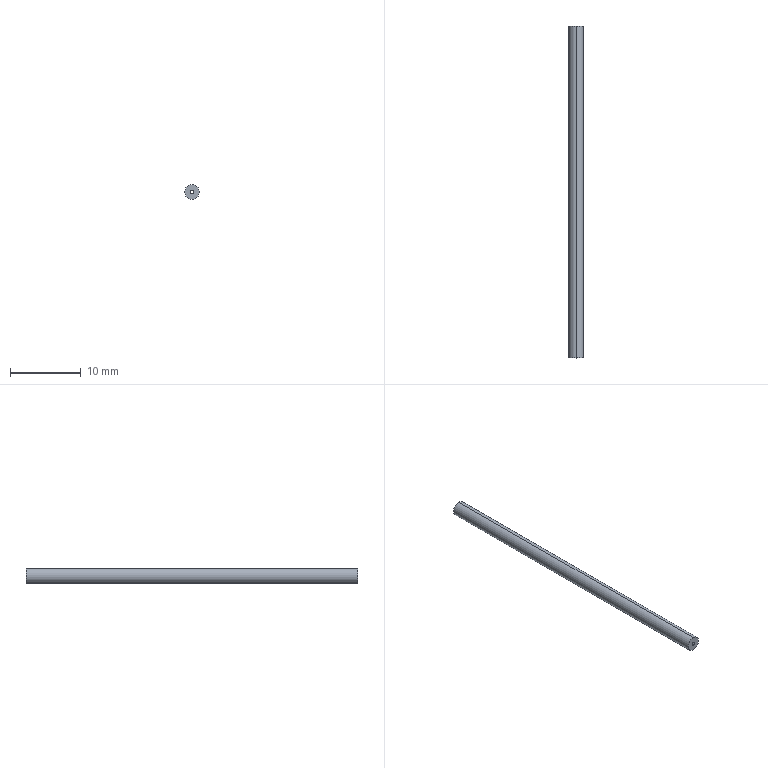Part | SolidWorks | features Revolution 1 | 1 solid | 6 faces | box 2.1 x 47 x 2.1 mm | volume 153.561 mm3 | cylinder 4 | plane 2 | commonest cylinder face diameters 0.5 x2 2.1 x2
STEP:
#1=CARTESIAN_POINT('',(0.,47.,0.25));
#2=VERTEX_POINT('',#1);
#3=CARTESIAN_POINT('',(0.,47.,-0.25));
#4=VERTEX_POINT('',#3);
#5=CARTESIAN_POINT('',(0.,47.,0.));
#6=DIRECTION('',(0.,-1.,0.));
#7=DIRECTION('',(0.,0.,-1.));
#8=AXIS2_PLACEMENT_3D('',#5,#6,#7);
#9=CIRCLE('',#8,0.25);
#10=EDGE_CURVE('',#2,#4,#9,.T.);
#11=ORIENTED_EDGE('',*,*,#10,.F.);
#12=CARTESIAN_POINT('',(0.,0.,0.25));
#13=VERTEX_POINT('',#12);
#14=CARTESIAN_POINT('',(0.,-3.568,0.25));
#15=DIRECTION('',(0.,-1.,0.));
#16=VECTOR('',#15,1000.);
#17=LINE('',#14,#16);
#18=EDGE_CURVE('',#2,#13,#17,.T.);
#19=ORIENTED_EDGE('',*,*,#18,.T.);
#20=CARTESIAN_POINT('',(0.,0.,-0.25));
#21=VERTEX_POINT('',#20);
#22=CARTESIAN_POINT('',(0.,0.,0.));
#23=DIRECTION('',(0.,-1.,0.));
#24=DIRECTION('',(0.,0.,-1.));
#25=AXIS2_PLACEMENT_3D('',#22,#23,#24);
#26=CIRCLE('',#25,0.25);
#27=EDGE_CURVE('',#13,#21,#26,.T.);
#28=ORIENTED_EDGE('',*,*,#27,.T.);
#29=CARTESIAN_POINT('',(0.,-3.568,-0.25));
#30=DIRECTION('',(0.,-1.,0.));
#31=VECTOR('',#30,1000.);
#32=LINE('',#29,#31);
#33=EDGE_CURVE('',#4,#21,#32,.T.);
#34=ORIENTED_EDGE('',*,*,#33,.F.);
#35=EDGE_LOOP('',(#11,#19,#28,#34));
#36=FACE_OUTER_BOUND('',#35,.T.);
#37=CARTESIAN_POINT('',(0.,-3.568,0.));
#38=DIRECTION('',(0.,-1.,0.));
#39=DIRECTION('',(0.,0.,-1.));
#40=AXIS2_PLACEMENT_3D('',#37,#38,#39);
#41=CYLINDRICAL_SURFACE('',#40,0.25);
#42=ADVANCED_FACE('',(#36),#41,.F.);
#43=CARTESIAN_POINT('',(0.,47.,-1.05));
#44=VERTEX_POINT('',#43);
#45=CARTESIAN_POINT('',(0.,47.,1.05));
#46=VERTEX_POINT('',#45);
#47=CARTESIAN_POINT('',(0.,47.,0.));
#48=DIRECTION('',(0.,-1.,0.));
#49=DIRECTION('',(0.,0.,-1.));
#50=AXIS2_PLACEMENT_3D('',#47,#48,#49);
#51=CIRCLE('',#50,1.05);
#52=EDGE_CURVE('',#44,#46,#51,.T.);
#53=ORIENTED_EDGE('',*,*,#52,.T.);
#54=CARTESIAN_POINT('',(0.,0.,1.05));
#55=VERTEX_POINT('',#54);
#56=CARTESIAN_POINT('',(0.,-3.568,1.05));
#57=DIRECTION('',(0.,-1.,0.));
#58=VECTOR('',#57,1000.);
#59=LINE('',#56,#58);
#60=EDGE_CURVE('',#46,#55,#59,.T.);
#61=ORIENTED_EDGE('',*,*,#60,.T.);
#62=CARTESIAN_POINT('',(0.,0.,-1.05));
#63=VERTEX_POINT('',#62);
#64=CARTESIAN_POINT('',(0.,0.,0.));
#65=DIRECTION('',(0.,-1.,0.));
#66=DIRECTION('',(0.,0.,-1.));
#67=AXIS2_PLACEMENT_3D('',#64,#65,#66);
#68=CIRCLE('',#67,1.05);
#69=EDGE_CURVE('',#63,#55,#68,.T.);
#70=ORIENTED_EDGE('',*,*,#69,.F.);
#71=CARTESIAN_POINT('',(0.,-3.568,-1.05));
#72=DIRECTION('',(0.,-1.,0.));
#73=VECTOR('',#72,1000.);
#74=LINE('',#71,#73);
#75=EDGE_CURVE('',#44,#63,#74,.T.);
#76=ORIENTED_EDGE('',*,*,#75,.F.);
#77=EDGE_LOOP('',(#53,#61,#70,#76));
#78=FACE_OUTER_BOUND('',#77,.T.);
#79=CARTESIAN_POINT('',(0.,-3.568,0.));
#80=DIRECTION('',(0.,-1.,0.));
#81=DIRECTION('',(0.,0.,-1.));
#82=AXIS2_PLACEMENT_3D('',#79,#80,#81);
#83=CYLINDRICAL_SURFACE('',#82,1.05);
#84=ADVANCED_FACE('',(#78),#83,.T.);
#85=ORIENTED_EDGE('',*,*,#60,.F.);
#86=CARTESIAN_POINT('',(0.,47.,0.));
#87=DIRECTION('',(0.,-1.,0.));
#88=DIRECTION('',(0.,0.,-1.));
#89=AXIS2_PLACEMENT_3D('',#86,#87,#88);
#90=CIRCLE('',#89,1.05);
#91=EDGE_CURVE('',#46,#44,#90,.T.);
#92=ORIENTED_EDGE('',*,*,#91,.T.);
#93=ORIENTED_EDGE('',*,*,#75,.T.);
#94=CARTESIAN_POINT('',(0.,0.,0.));
#95=DIRECTION('',(0.,-1.,0.));
#96=DIRECTION('',(0.,0.,-1.));
#97=AXIS2_PLACEMENT_3D('',#94,#95,#96);
#98=CIRCLE('',#97,1.05);
#99=EDGE_CURVE('',#55,#63,#98,.T.);
#100=ORIENTED_EDGE('',*,*,#99,.F.);
#101=EDGE_LOOP('',(#85,#92,#93,#100));
#102=FACE_OUTER_BOUND('',#101,.T.);
#103=CARTESIAN_POINT('',(0.,-3.568,0.));
#104=DIRECTION('',(0.,-1.,0.));
#105=DIRECTION('',(0.,0.,-1.));
#106=AXIS2_PLACEMENT_3D('',#103,#104,#105);
#107=CYLINDRICAL_SURFACE('',#106,1.05);
#108=ADVANCED_FACE('',(#102),#107,.T.);
#109=ORIENTED_EDGE('',*,*,#52,.F.);
#110=ORIENTED_EDGE('',*,*,#91,.F.);
#111=EDGE_LOOP('',(#109,#110));
#112=FACE_OUTER_BOUND('',#111,.T.);
#113=CARTESIAN_POINT('',(0.,47.,0.));
#114=DIRECTION('',(0.,-1.,0.));
#115=DIRECTION('',(0.,0.,-1.));
#116=AXIS2_PLACEMENT_3D('',#113,#114,#115);
#117=CIRCLE('',#116,0.25);
#118=EDGE_CURVE('',#4,#2,#117,.T.);
#119=ORIENTED_EDGE('',*,*,#118,.T.);
#120=ORIENTED_EDGE('',*,*,#10,.T.);
#121=EDGE_LOOP('',(#119,#120));
#122=FACE_BOUND('',#121,.T.);
#123=CARTESIAN_POINT('',(-1.05,47.,0.));
#124=DIRECTION('',(0.,-1.,0.));
#125=DIRECTION('',(0.,0.,-1.));
#126=AXIS2_PLACEMENT_3D('',#123,#124,#125);
#127=PLANE('',#126);
#128=ADVANCED_FACE('',(#112,#122),#127,.F.);
#129=ORIENTED_EDGE('',*,*,#18,.F.);
#130=ORIENTED_EDGE('',*,*,#118,.F.);
#131=ORIENTED_EDGE('',*,*,#33,.T.);
#132=CARTESIAN_POINT('',(0.,0.,0.));
#133=DIRECTION('',(0.,-1.,0.));
#134=DIRECTION('',(0.,0.,-1.));
#135=AXIS2_PLACEMENT_3D('',#132,#133,#134);
#136=CIRCLE('',#135,0.25);
#137=EDGE_CURVE('',#21,#13,#136,.T.);
#138=ORIENTED_EDGE('',*,*,#137,.T.);
#139=EDGE_LOOP('',(#129,#130,#131,#138));
#140=FACE_OUTER_BOUND('',#139,.T.);
#141=CARTESIAN_POINT('',(0.,-3.568,0.));
#142=DIRECTION('',(0.,-1.,0.));
#143=DIRECTION('',(0.,0.,-1.));
#144=AXIS2_PLACEMENT_3D('',#141,#142,#143);
#145=CYLINDRICAL_SURFACE('',#144,0.25);
#146=ADVANCED_FACE('',(#140),#145,.F.);
#147=ORIENTED_EDGE('',*,*,#137,.F.);
#148=ORIENTED_EDGE('',*,*,#27,.F.);
#149=EDGE_LOOP('',(#147,#148));
#150=FACE_BOUND('',#149,.T.);
#151=ORIENTED_EDGE('',*,*,#69,.T.);
#152=ORIENTED_EDGE('',*,*,#99,.T.);
#153=EDGE_LOOP('',(#151,#152));
#154=FACE_OUTER_BOUND('',#153,.T.);
#155=CARTESIAN_POINT('',(-1.05,0.,0.));
#156=DIRECTION('',(0.,1.,0.));
#157=DIRECTION('',(0.,0.,1.));
#158=AXIS2_PLACEMENT_3D('',#155,#156,#157);
#159=PLANE('',#158);
#160=ADVANCED_FACE('',(#150,#154),#159,.F.);
#161=CLOSED_SHELL('',(#42,#84,#108,#128,#146,#160));
#162=MANIFOLD_SOLID_BREP('',#161);
#163=CARTESIAN_POINT('',(0.,0.,0.));
#164=DIRECTION('',(0.,0.,1.));
#165=DIRECTION('',(1.,0.,0.));
#166=AXIS2_PLACEMENT_3D('',#163,#164,#165);
#167=(LENGTH_UNIT()NAMED_UNIT(*)SI_UNIT(.MILLI.,.METRE.));
#168=UNCERTAINTY_MEASURE_WITH_UNIT(LENGTH_MEASURE(0.00001),#167,'','');
#169=(NAMED_UNIT(*)PLANE_ANGLE_UNIT()SI_UNIT($,.RADIAN.));
#170=(NAMED_UNIT(*)SI_UNIT($,.STERADIAN.)SOLID_ANGLE_UNIT());
#171=(GEOMETRIC_REPRESENTATION_CONTEXT(3)GLOBAL_UNCERTAINTY_ASSIGNED_CONTEXT((#168))GLOBAL_UNIT_ASSIGNED_CONTEXT((#167,#169,#170))REPRESENTATION_CONTEXT('',''));
#172=ADVANCED_BREP_SHAPE_REPRESENTATION('',(#162,#166),#171);